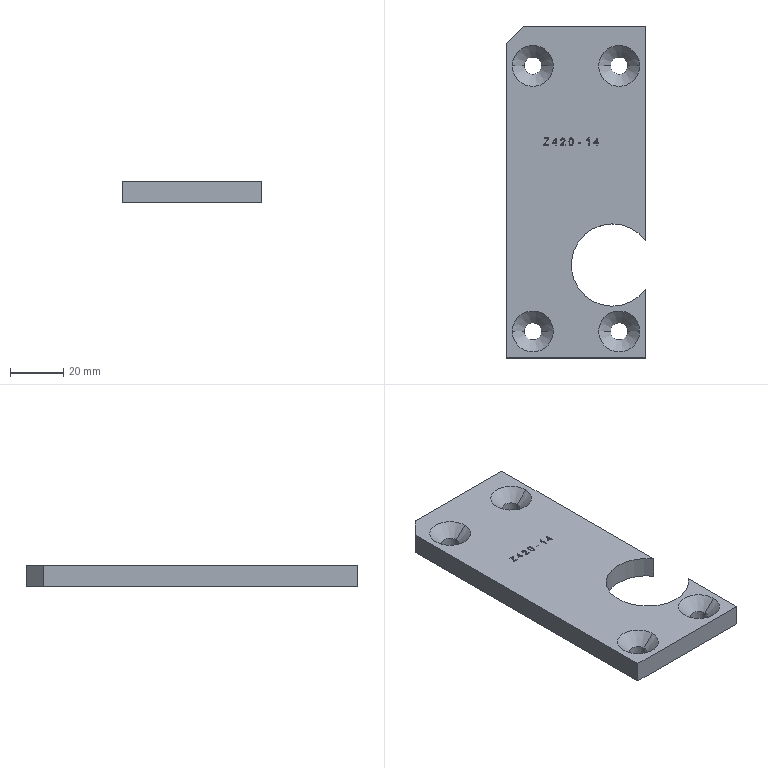Part | Creo | 1 solid | 130 faces | box 52.5 x 125 x 8 mm | volume 44338 mm3 | plane 62 | other 49 | cylinder 11 | cone 8 | commonest cylinder face diameters 6.5 x8 2.427 x1 31 x1 38.273 x1